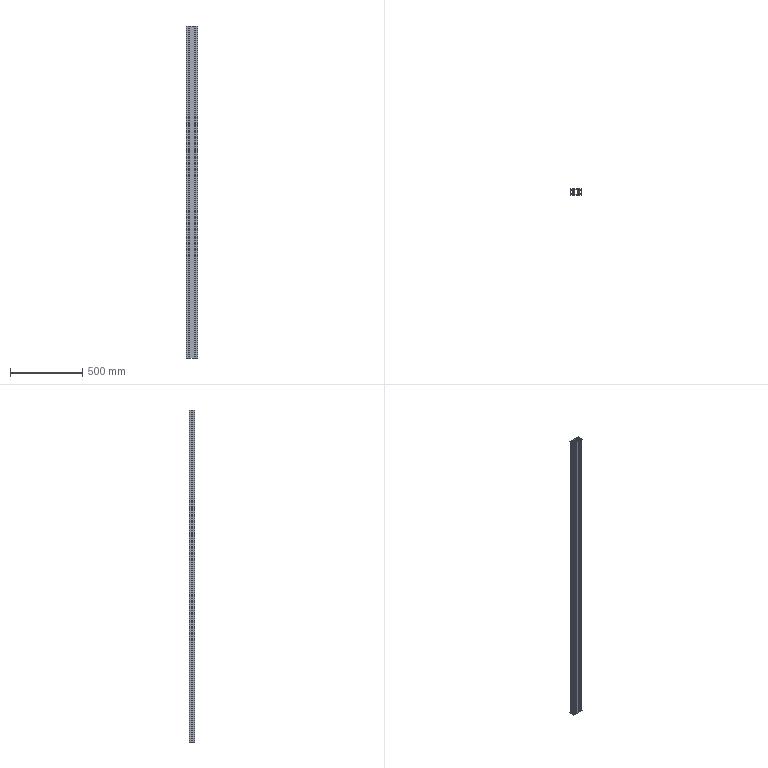Part | SolidWorks | features MBimport 1 | 1 solid | 248 faces | box 80 x 40 x 2300 mm | volume 2517050 mm3 | plane 182 | cylinder 66 | commonest cylinder face diameters 0.6 x16 1 x12 1.5 x12 2 x12 6.8 x10 4 x4